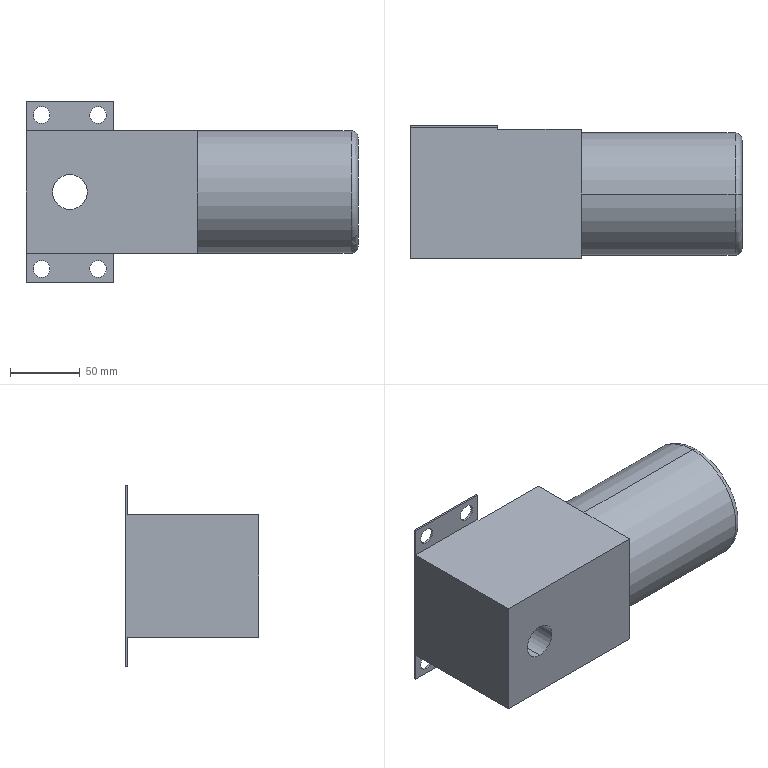Part | SolidWorks | features ICE 5, Extrusion 1, Fillet 1 | 1 solid | 28 faces | box 238.5 x 96 x 130.5 mm | volume 1680517 mm3 | plane 14 | cylinder 12 | torus 2 | commonest cylinder face diameters 12 x8 25 x2 88 x2
STEP:
#1=CARTESIAN_POINT('',(202.,-48.,44.));
#2=VERTEX_POINT('',#1);
#3=CARTESIAN_POINT('',(202.,-48.,-44.));
#4=VERTEX_POINT('',#3);
#5=CARTESIAN_POINT('',(202.,-48.,0.));
#6=DIRECTION('',(-1.,0.,0.));
#7=DIRECTION('',(0.,0.,-1.));
#8=AXIS2_PLACEMENT_3D('',#5,#6,#7);
#9=CIRCLE('',#8,44.);
#10=EDGE_CURVE('',#2,#4,#9,.T.);
#11=ORIENTED_EDGE('',*,*,#10,.F.);
#12=CARTESIAN_POINT('',(207.,-48.,39.));
#13=VERTEX_POINT('',#12);
#14=CARTESIAN_POINT('',(202.,-48.,39.));
#15=DIRECTION('',(0.,1.,0.));
#16=DIRECTION('',(0.,0.,1.));
#17=AXIS2_PLACEMENT_3D('',#14,#15,#16);
#18=CIRCLE('',#17,5.);
#19=EDGE_CURVE('',#2,#13,#18,.T.);
#20=ORIENTED_EDGE('',*,*,#19,.T.);
#21=CARTESIAN_POINT('',(207.,-48.,-39.));
#22=VERTEX_POINT('',#21);
#23=CARTESIAN_POINT('',(207.,-48.,0.));
#24=DIRECTION('',(1.,0.,0.));
#25=DIRECTION('',(0.,0.,-1.));
#26=AXIS2_PLACEMENT_3D('',#23,#24,#25);
#27=CIRCLE('',#26,39.);
#28=EDGE_CURVE('',#22,#13,#27,.T.);
#29=ORIENTED_EDGE('',*,*,#28,.F.);
#30=CARTESIAN_POINT('',(202.,-48.,-39.));
#31=DIRECTION('',(0.,-1.,0.));
#32=DIRECTION('',(0.,0.,-1.));
#33=AXIS2_PLACEMENT_3D('',#30,#31,#32);
#34=CIRCLE('',#33,5.);
#35=EDGE_CURVE('',#4,#22,#34,.T.);
#36=ORIENTED_EDGE('',*,*,#35,.F.);
#37=EDGE_LOOP('',(#11,#20,#29,#36));
#38=FACE_OUTER_BOUND('',#37,.T.);
#39=CARTESIAN_POINT('',(202.,-48.,0.));
#40=DIRECTION('',(1.,0.,0.));
#41=DIRECTION('',(0.,0.,-1.));
#42=AXIS2_PLACEMENT_3D('',#39,#40,#41);
#43=TOROIDAL_SURFACE('',#42,39.,5.);
#44=ADVANCED_FACE('',(#38),#43,.T.);
#45=CARTESIAN_POINT('',(0.,-94.5,-12.5));
#46=VERTEX_POINT('',#45);
#47=CARTESIAN_POINT('',(0.,-94.5,12.5));
#48=VERTEX_POINT('',#47);
#49=CARTESIAN_POINT('',(0.,-94.5,0.));
#50=DIRECTION('',(0.,1.,0.));
#51=DIRECTION('',(0.,0.,1.));
#52=AXIS2_PLACEMENT_3D('',#49,#50,#51);
#53=CIRCLE('',#52,12.5);
#54=EDGE_CURVE('',#46,#48,#53,.T.);
#55=ORIENTED_EDGE('',*,*,#54,.F.);
#56=CARTESIAN_POINT('',(0.,1.5,-12.5));
#57=VERTEX_POINT('',#56);
#58=CARTESIAN_POINT('',(0.,-94.5,-12.5));
#59=DIRECTION('',(0.,1.,0.));
#60=VECTOR('',#59,1000.);
#61=LINE('',#58,#60);
#62=EDGE_CURVE('',#46,#57,#61,.T.);
#63=ORIENTED_EDGE('',*,*,#62,.T.);
#64=CARTESIAN_POINT('',(0.,1.5,12.5));
#65=VERTEX_POINT('',#64);
#66=CARTESIAN_POINT('',(0.,1.5,0.));
#67=DIRECTION('',(0.,1.,0.));
#68=DIRECTION('',(0.,0.,1.));
#69=AXIS2_PLACEMENT_3D('',#66,#67,#68);
#70=CIRCLE('',#69,12.5);
#71=EDGE_CURVE('',#57,#65,#70,.T.);
#72=ORIENTED_EDGE('',*,*,#71,.T.);
#73=CARTESIAN_POINT('',(0.,-94.5,12.5));
#74=DIRECTION('',(0.,1.,0.));
#75=VECTOR('',#74,1000.);
#76=LINE('',#73,#75);
#77=EDGE_CURVE('',#48,#65,#76,.T.);
#78=ORIENTED_EDGE('',*,*,#77,.F.);
#79=EDGE_LOOP('',(#55,#63,#72,#78));
#80=FACE_OUTER_BOUND('',#79,.T.);
#81=CARTESIAN_POINT('',(0.,-94.5,0.));
#82=DIRECTION('',(0.,1.,0.));
#83=DIRECTION('',(0.,0.,1.));
#84=AXIS2_PLACEMENT_3D('',#81,#82,#83);
#85=CYLINDRICAL_SURFACE('',#84,12.5);
#86=ADVANCED_FACE('',(#80),#85,.F.);
#87=CARTESIAN_POINT('',(20.25,0.,49.25));
#88=VERTEX_POINT('',#87);
#89=CARTESIAN_POINT('',(20.25,0.,61.25));
#90=VERTEX_POINT('',#89);
#91=CARTESIAN_POINT('',(20.25,0.,55.25));
#92=DIRECTION('',(0.,1.,0.));
#93=DIRECTION('',(0.,0.,1.));
#94=AXIS2_PLACEMENT_3D('',#91,#92,#93);
#95=CIRCLE('',#94,6.);
#96=EDGE_CURVE('',#88,#90,#95,.T.);
#97=ORIENTED_EDGE('',*,*,#96,.F.);
#98=CARTESIAN_POINT('',(20.25,1.5,49.25));
#99=VERTEX_POINT('',#98);
#100=CARTESIAN_POINT('',(20.25,-94.5,49.25));
#101=DIRECTION('',(0.,1.,0.));
#102=VECTOR('',#101,1000.);
#103=LINE('',#100,#102);
#104=EDGE_CURVE('',#88,#99,#103,.T.);
#105=ORIENTED_EDGE('',*,*,#104,.T.);
#106=CARTESIAN_POINT('',(20.25,1.5,61.25));
#107=VERTEX_POINT('',#106);
#108=CARTESIAN_POINT('',(20.25,1.5,55.25));
#109=DIRECTION('',(0.,1.,0.));
#110=DIRECTION('',(0.,0.,1.));
#111=AXIS2_PLACEMENT_3D('',#108,#109,#110);
#112=CIRCLE('',#111,6.);
#113=EDGE_CURVE('',#99,#107,#112,.T.);
#114=ORIENTED_EDGE('',*,*,#113,.T.);
#115=CARTESIAN_POINT('',(20.25,-94.5,61.25));
#116=DIRECTION('',(0.,1.,0.));
#117=VECTOR('',#116,1000.);
#118=LINE('',#115,#117);
#119=EDGE_CURVE('',#90,#107,#118,.T.);
#120=ORIENTED_EDGE('',*,*,#119,.F.);
#121=EDGE_LOOP('',(#97,#105,#114,#120));
#122=FACE_OUTER_BOUND('',#121,.T.);
#123=CARTESIAN_POINT('',(20.25,-94.5,55.25));
#124=DIRECTION('',(0.,1.,0.));
#125=DIRECTION('',(0.,0.,1.));
#126=AXIS2_PLACEMENT_3D('',#123,#124,#125);
#127=CYLINDRICAL_SURFACE('',#126,6.);
#128=ADVANCED_FACE('',(#122),#127,.F.);
#129=CARTESIAN_POINT('',(-20.25,0.,49.25));
#130=VERTEX_POINT('',#129);
#131=CARTESIAN_POINT('',(-20.25,0.,61.25));
#132=VERTEX_POINT('',#131);
#133=CARTESIAN_POINT('',(-20.25,0.,55.25));
#134=DIRECTION('',(0.,1.,0.));
#135=DIRECTION('',(0.,0.,1.));
#136=AXIS2_PLACEMENT_3D('',#133,#134,#135);
#137=CIRCLE('',#136,6.);
#138=EDGE_CURVE('',#130,#132,#137,.T.);
#139=ORIENTED_EDGE('',*,*,#138,.F.);
#140=CARTESIAN_POINT('',(-20.25,1.5,49.25));
#141=VERTEX_POINT('',#140);
#142=CARTESIAN_POINT('',(-20.25,-94.5,49.25));
#143=DIRECTION('',(0.,1.,0.));
#144=VECTOR('',#143,1000.);
#145=LINE('',#142,#144);
#146=EDGE_CURVE('',#130,#141,#145,.T.);
#147=ORIENTED_EDGE('',*,*,#146,.T.);
#148=CARTESIAN_POINT('',(-20.25,1.5,61.25));
#149=VERTEX_POINT('',#148);
#150=CARTESIAN_POINT('',(-20.25,1.5,55.25));
#151=DIRECTION('',(0.,1.,0.));
#152=DIRECTION('',(0.,0.,1.));
#153=AXIS2_PLACEMENT_3D('',#150,#151,#152);
#154=CIRCLE('',#153,6.);
#155=EDGE_CURVE('',#141,#149,#154,.T.);
#156=ORIENTED_EDGE('',*,*,#155,.T.);
#157=CARTESIAN_POINT('',(-20.25,-94.5,61.25));
#158=DIRECTION('',(0.,1.,0.));
#159=VECTOR('',#158,1000.);
#160=LINE('',#157,#159);
#161=EDGE_CURVE('',#132,#149,#160,.T.);
#162=ORIENTED_EDGE('',*,*,#161,.F.);
#163=EDGE_LOOP('',(#139,#147,#156,#162));
#164=FACE_OUTER_BOUND('',#163,.T.);
#165=CARTESIAN_POINT('',(-20.25,-94.5,55.25));
#166=DIRECTION('',(0.,1.,0.));
#167=DIRECTION('',(0.,0.,1.));
#168=AXIS2_PLACEMENT_3D('',#165,#166,#167);
#169=CYLINDRICAL_SURFACE('',#168,6.);
#170=ADVANCED_FACE('',(#164),#169,.F.);
#171=CARTESIAN_POINT('',(20.25,0.,-61.25));
#172=VERTEX_POINT('',#171);
#173=CARTESIAN_POINT('',(20.25,0.,-49.25));
#174=VERTEX_POINT('',#173);
#175=CARTESIAN_POINT('',(20.25,0.,-55.25));
#176=DIRECTION('',(0.,1.,0.));
#177=DIRECTION('',(0.,0.,1.));
#178=AXIS2_PLACEMENT_3D('',#175,#176,#177);
#179=CIRCLE('',#178,6.);
#180=EDGE_CURVE('',#172,#174,#179,.T.);
#181=ORIENTED_EDGE('',*,*,#180,.F.);
#182=CARTESIAN_POINT('',(20.25,1.5,-61.25));
#183=VERTEX_POINT('',#182);
#184=CARTESIAN_POINT('',(20.25,-94.5,-61.25));
#185=DIRECTION('',(0.,1.,0.));
#186=VECTOR('',#185,1000.);
#187=LINE('',#184,#186);
#188=EDGE_CURVE('',#172,#183,#187,.T.);
#189=ORIENTED_EDGE('',*,*,#188,.T.);
#190=CARTESIAN_POINT('',(20.25,1.5,-49.25));
#191=VERTEX_POINT('',#190);
#192=CARTESIAN_POINT('',(20.25,1.5,-55.25));
#193=DIRECTION('',(0.,1.,0.));
#194=DIRECTION('',(0.,0.,1.));
#195=AXIS2_PLACEMENT_3D('',#192,#193,#194);
#196=CIRCLE('',#195,6.);
#197=EDGE_CURVE('',#183,#191,#196,.T.);
#198=ORIENTED_EDGE('',*,*,#197,.T.);
#199=CARTESIAN_POINT('',(20.25,-94.5,-49.25));
#200=DIRECTION('',(0.,1.,0.));
#201=VECTOR('',#200,1000.);
#202=LINE('',#199,#201);
#203=EDGE_CURVE('',#174,#191,#202,.T.);
#204=ORIENTED_EDGE('',*,*,#203,.F.);
#205=EDGE_LOOP('',(#181,#189,#198,#204));
#206=FACE_OUTER_BOUND('',#205,.T.);
#207=CARTESIAN_POINT('',(20.25,-94.5,-55.25));
#208=DIRECTION('',(0.,1.,0.));
#209=DIRECTION('',(0.,0.,1.));
#210=AXIS2_PLACEMENT_3D('',#207,#208,#209);
#211=CYLINDRICAL_SURFACE('',#210,6.);
#212=ADVANCED_FACE('',(#206),#211,.F.);
#213=CARTESIAN_POINT('',(-20.25,0.,-61.25));
#214=VERTEX_POINT('',#213);
#215=CARTESIAN_POINT('',(-20.25,0.,-49.25));
#216=VERTEX_POINT('',#215);
#217=CARTESIAN_POINT('',(-20.25,0.,-55.25));
#218=DIRECTION('',(0.,1.,0.));
#219=DIRECTION('',(0.,0.,1.));
#220=AXIS2_PLACEMENT_3D('',#217,#218,#219);
#221=CIRCLE('',#220,6.);
#222=EDGE_CURVE('',#214,#216,#221,.T.);
#223=ORIENTED_EDGE('',*,*,#222,.F.);
#224=CARTESIAN_POINT('',(-20.25,1.5,-61.25));
#225=VERTEX_POINT('',#224);
#226=CARTESIAN_POINT('',(-20.25,-94.5,-61.25));
#227=DIRECTION('',(0.,1.,0.));
#228=VECTOR('',#227,1000.);
#229=LINE('',#226,#228);
#230=EDGE_CURVE('',#214,#225,#229,.T.);
#231=ORIENTED_EDGE('',*,*,#230,.T.);
#232=CARTESIAN_POINT('',(-20.25,1.5,-49.25));
#233=VERTEX_POINT('',#232);
#234=CARTESIAN_POINT('',(-20.25,1.5,-55.25));
#235=DIRECTION('',(0.,1.,0.));
#236=DIRECTION('',(0.,0.,1.));
#237=AXIS2_PLACEMENT_3D('',#234,#235,#236);
#238=CIRCLE('',#237,6.);
#239=EDGE_CURVE('',#225,#233,#238,.T.);
#240=ORIENTED_EDGE('',*,*,#239,.T.);
#241=CARTESIAN_POINT('',(-20.25,-94.5,-49.25));
#242=DIRECTION('',(0.,1.,0.));
#243=VECTOR('',#242,1000.);
#244=LINE('',#241,#243);
#245=EDGE_CURVE('',#216,#233,#244,.T.);
#246=ORIENTED_EDGE('',*,*,#245,.F.);
#247=EDGE_LOOP('',(#223,#231,#240,#246));
#248=FACE_OUTER_BOUND('',#247,.T.);
#249=CARTESIAN_POINT('',(-20.25,-94.5,-55.25));
#250=DIRECTION('',(0.,1.,0.));
#251=DIRECTION('',(0.,0.,1.));
#252=AXIS2_PLACEMENT_3D('',#249,#250,#251);
#253=CYLINDRICAL_SURFACE('',#252,6.);
#254=ADVANCED_FACE('',(#248),#253,.F.);
#255=ORIENTED_EDGE('',*,*,#10,.T.);
#256=CARTESIAN_POINT('',(91.5,-48.,-44.));
#257=VERTEX_POINT('',#256);
#258=CARTESIAN_POINT('',(207.,-48.,-44.));
#259=DIRECTION('',(-1.,0.,0.));
#260=VECTOR('',#259,1000.);
#261=LINE('',#258,#260);
#262=EDGE_CURVE('',#4,#257,#261,.T.);
#263=ORIENTED_EDGE('',*,*,#262,.T.);
#264=CARTESIAN_POINT('',(91.5,-48.,44.));
#265=VERTEX_POINT('',#264);
#266=CARTESIAN_POINT('',(91.5,-48.,0.));
#267=DIRECTION('',(1.,0.,0.));
#268=DIRECTION('',(0.,0.,-1.));
#269=AXIS2_PLACEMENT_3D('',#266,#267,#268);
#270=CIRCLE('',#269,44.);
#271=EDGE_CURVE('',#257,#265,#270,.T.);
#272=ORIENTED_EDGE('',*,*,#271,.T.);
#273=CARTESIAN_POINT('',(207.,-48.,44.));
#274=DIRECTION('',(-1.,0.,0.));
#275=VECTOR('',#274,1000.);
#276=LINE('',#273,#275);
#277=EDGE_CURVE('',#2,#265,#276,.T.);
#278=ORIENTED_EDGE('',*,*,#277,.F.);
#279=EDGE_LOOP('',(#255,#263,#272,#278));
#280=FACE_OUTER_BOUND('',#279,.T.);
#281=CARTESIAN_POINT('',(207.,-48.,0.));
#282=DIRECTION('',(-1.,0.,0.));
#283=DIRECTION('',(0.,0.,1.));
#284=AXIS2_PLACEMENT_3D('',#281,#282,#283);
#285=CYLINDRICAL_SURFACE('',#284,44.);
#286=ADVANCED_FACE('',(#280),#285,.T.);
#287=CARTESIAN_POINT('',(31.5,-1.5,-44.));
#288=VERTEX_POINT('',#287);
#289=CARTESIAN_POINT('',(31.5,-1.5,44.));
#290=VERTEX_POINT('',#289);
#291=CARTESIAN_POINT('',(31.5,-1.5,-65.25));
#292=DIRECTION('',(0.,0.,1.));
#293=VECTOR('',#292,1000.);
#294=LINE('',#291,#293);
#295=EDGE_CURVE('',#288,#290,#294,.T.);
#296=ORIENTED_EDGE('',*,*,#295,.F.);
#297=CARTESIAN_POINT('',(31.5,0.,-44.));
#298=VERTEX_POINT('',#297);
#299=CARTESIAN_POINT('',(31.5,-3.,-44.));
#300=DIRECTION('',(0.,1.,0.));
#301=VECTOR('',#300,1000.);
#302=LINE('',#299,#301);
#303=EDGE_CURVE('',#288,#298,#302,.T.);
#304=ORIENTED_EDGE('',*,*,#303,.T.);
#305=CARTESIAN_POINT('',(31.5,0.,-65.25));
#306=VERTEX_POINT('',#305);
#307=CARTESIAN_POINT('',(31.5,0.,-65.25));
#308=DIRECTION('',(0.,0.,-1.));
#309=VECTOR('',#308,1000.);
#310=LINE('',#307,#309);
#311=EDGE_CURVE('',#298,#306,#310,.T.);
#312=ORIENTED_EDGE('',*,*,#311,.T.);
#313=CARTESIAN_POINT('',(31.5,1.5,-65.25));
#314=VERTEX_POINT('',#313);
#315=CARTESIAN_POINT('',(31.5,1.5,-65.25));
#316=DIRECTION('',(0.,-1.,0.));
#317=VECTOR('',#316,1000.);
#318=LINE('',#315,#317);
#319=EDGE_CURVE('',#314,#306,#318,.T.);
#320=ORIENTED_EDGE('',*,*,#319,.F.);
#321=CARTESIAN_POINT('',(31.5,1.5,65.25));
#322=VERTEX_POINT('',#321);
#323=CARTESIAN_POINT('',(31.5,1.5,-65.25));
#324=DIRECTION('',(0.,0.,-1.));
#325=VECTOR('',#324,1000.);
#326=LINE('',#323,#325);
#327=EDGE_CURVE('',#322,#314,#326,.T.);
#328=ORIENTED_EDGE('',*,*,#327,.F.);
#329=CARTESIAN_POINT('',(31.5,0.,65.25));
#330=VERTEX_POINT('',#329);
#331=CARTESIAN_POINT('',(31.5,1.5,65.25));
#332=DIRECTION('',(0.,-1.,0.));
#333=VECTOR('',#332,1000.);
#334=LINE('',#331,#333);
#335=EDGE_CURVE('',#322,#330,#334,.T.);
#336=ORIENTED_EDGE('',*,*,#335,.T.);
#337=CARTESIAN_POINT('',(31.5,0.,44.));
#338=VERTEX_POINT('',#337);
#339=CARTESIAN_POINT('',(31.5,0.,-65.25));
#340=DIRECTION('',(0.,0.,-1.));
#341=VECTOR('',#340,1000.);
#342=LINE('',#339,#341);
#343=EDGE_CURVE('',#330,#338,#342,.T.);
#344=ORIENTED_EDGE('',*,*,#343,.T.);
#345=CARTESIAN_POINT('',(31.5,-3.,44.));
#346=DIRECTION('',(0.,1.,0.));
#347=VECTOR('',#346,1000.);
#348=LINE('',#345,#347);
#349=EDGE_CURVE('',#290,#338,#348,.T.);
#350=ORIENTED_EDGE('',*,*,#349,.F.);
#351=EDGE_LOOP('',(#296,#304,#312,#320,#328,#336,#344,#350));
#352=FACE_OUTER_BOUND('',#351,.T.);
#353=CARTESIAN_POINT('',(31.5,1.5,-65.25));
#354=DIRECTION('',(-1.,0.,0.));
#355=DIRECTION('',(0.,0.,1.));
#356=AXIS2_PLACEMENT_3D('',#353,#354,#355);
#357=PLANE('',#356);
#358=ADVANCED_FACE('',(#352),#357,.F.);
#359=CARTESIAN_POINT('',(20.25,0.,55.25));
#360=DIRECTION('',(0.,1.,0.));
#361=DIRECTION('',(0.,0.,1.));
#362=AXIS2_PLACEMENT_3D('',#359,#360,#361);
#363=CIRCLE('',#362,6.);
#364=EDGE_CURVE('',#90,#88,#363,.T.);
#365=ORIENTED_EDGE('',*,*,#364,.T.);
#366=ORIENTED_EDGE('',*,*,#96,.T.);
#367=EDGE_LOOP('',(#365,#366));
#368=FACE_BOUND('',#367,.T.);
#369=CARTESIAN_POINT('',(-20.25,0.,55.25));
#370=DIRECTION('',(0.,1.,0.));
#371=DIRECTION('',(0.,0.,1.));
#372=AXIS2_PLACEMENT_3D('',#369,#370,#371);
#373=CIRCLE('',#372,6.);
#374=EDGE_CURVE('',#132,#130,#373,.T.);
#375=ORIENTED_EDGE('',*,*,#374,.T.);
#376=ORIENTED_EDGE('',*,*,#138,.T.);
#377=EDGE_LOOP('',(#375,#376));
#378=FACE_BOUND('',#377,.T.);
#379=CARTESIAN_POINT('',(-31.5,0.,44.));
#380=VERTEX_POINT('',#379);
#381=CARTESIAN_POINT('',(-31.5,0.,44.));
#382=DIRECTION('',(-1.,0.,0.));
#383=VECTOR('',#382,1000.);
#384=LINE('',#381,#383);
#385=EDGE_CURVE('',#338,#380,#384,.T.);
#386=ORIENTED_EDGE('',*,*,#385,.F.);
#387=ORIENTED_EDGE('',*,*,#343,.F.);
#388=CARTESIAN_POINT('',(-31.5,0.,65.25));
#389=VERTEX_POINT('',#388);
#390=CARTESIAN_POINT('',(-31.5,0.,65.25));
#391=DIRECTION('',(1.,0.,0.));
#392=VECTOR('',#391,1000.);
#393=LINE('',#390,#392);
#394=EDGE_CURVE('',#389,#330,#393,.T.);
#395=ORIENTED_EDGE('',*,*,#394,.F.);
#396=CARTESIAN_POINT('',(-31.5,0.,-65.25));
#397=DIRECTION('',(0.,0.,1.));
#398=VECTOR('',#397,1000.);
#399=LINE('',#396,#398);
#400=EDGE_CURVE('',#380,#389,#399,.T.);
#401=ORIENTED_EDGE('',*,*,#400,.F.);
#402=EDGE_LOOP('',(#386,#387,#395,#401));
#403=FACE_OUTER_BOUND('',#402,.T.);
#404=CARTESIAN_POINT('',(0.,0.,0.));
#405=DIRECTION('',(0.,1.,0.));
#406=DIRECTION('',(0.,0.,1.));
#407=AXIS2_PLACEMENT_3D('',#404,#405,#406);
#408=PLANE('',#407);
#409=ADVANCED_FACE('',(#368,#378,#403),#408,.F.);
#410=CARTESIAN_POINT('',(20.25,0.,-55.25));
#411=DIRECTION('',(0.,1.,0.));
#412=DIRECTION('',(0.,0.,1.));
#413=AXIS2_PLACEMENT_3D('',#410,#411,#412);
#414=CIRCLE('',#413,6.);
#415=EDGE_CURVE('',#174,#172,#414,.T.);
#416=ORIENTED_EDGE('',*,*,#415,.T.);
#417=ORIENTED_EDGE('',*,*,#180,.T.);
#418=EDGE_LOOP('',(#416,#417));
#419=FACE_BOUND('',#418,.T.);
#420=CARTESIAN_POINT('',(-20.25,0.,-55.25));
#421=DIRECTION('',(0.,1.,0.));
#422=DIRECTION('',(0.,0.,1.));
#423=AXIS2_PLACEMENT_3D('',#420,#421,#422);
#424=CIRCLE('',#423,6.);
#425=EDGE_CURVE('',#216,#214,#424,.T.);
#426=ORIENTED_EDGE('',*,*,#425,.T.);
#427=ORIENTED_EDGE('',*,*,#222,.T.);
#428=EDGE_LOOP('',(#426,#427));
#429=FACE_BOUND('',#428,.T.);
#430=CARTESIAN_POINT('',(-31.5,0.,-44.));
#431=VERTEX_POINT('',#430);
#432=CARTESIAN_POINT('',(-31.5,0.,-44.));
#433=DIRECTION('',(1.,0.,0.));
#434=VECTOR('',#433,1000.);
#435=LINE('',#432,#434);
#436=EDGE_CURVE('',#431,#298,#435,.T.);
#437=ORIENTED_EDGE('',*,*,#436,.F.);
#438=CARTESIAN_POINT('',(-31.5,0.,-65.25));
#439=VERTEX_POINT('',#438);
#440=CARTESIAN_POINT('',(-31.5,0.,-65.25));
#441=DIRECTION('',(0.,0.,1.));
#442=VECTOR('',#441,1000.);
#443=LINE('',#440,#442);
#444=EDGE_CURVE('',#439,#431,#443,.T.);
#445=ORIENTED_EDGE('',*,*,#444,.F.);
#446=CARTESIAN_POINT('',(-31.5,0.,-65.25));
#447=DIRECTION('',(-1.,0.,0.));
#448=VECTOR('',#447,1000.);
#449=LINE('',#446,#448);
#450=EDGE_CURVE('',#306,#439,#449,.T.);
#451=ORIENTED_EDGE('',*,*,#450,.F.);
#452=ORIENTED_EDGE('',*,*,#311,.F.);
#453=EDGE_LOOP('',(#437,#445,#451,#452));
#454=FACE_OUTER_BOUND('',#453,.T.);
#455=CARTESIAN_POINT('',(0.,0.,0.));
#456=DIRECTION('',(0.,1.,0.));
#457=DIRECTION('',(0.,0.,1.));
#458=AXIS2_PLACEMENT_3D('',#455,#456,#457);
#459=PLANE('',#458);
#460=ADVANCED_FACE('',(#419,#429,#454),#459,.F.);
#461=ORIENTED_EDGE('',*,*,#450,.T.);
#462=CARTESIAN_POINT('',(-31.5,1.5,-65.25));
#463=VERTEX_POINT('',#462);
#464=CARTESIAN_POINT('',(-31.5,1.5,-65.25));
#465=DIRECTION('',(0.,-1.,0.));
#466=VECTOR('',#465,1000.);
#467=LINE('',#464,#466);
#468=EDGE_CURVE('',#463,#439,#467,.T.);
#469=ORIENTED_EDGE('',*,*,#468,.F.);
#470=CARTESIAN_POINT('',(-31.5,1.5,-65.25));
#471=DIRECTION('',(-1.,0.,0.));
#472=VECTOR('',#471,1000.);
#473=LINE('',#470,#472);
#474=EDGE_CURVE('',#314,#463,#473,.T.);
#475=ORIENTED_EDGE('',*,*,#474,.F.);
#476=ORIENTED_EDGE('',*,*,#319,.T.);
#477=EDGE_LOOP('',(#461,#469,#475,#476));
#478=FACE_OUTER_BOUND('',#477,.T.);
#479=CARTESIAN_POINT('',(-31.5,1.5,-65.25));
#480=DIRECTION('',(0.,0.,1.));
#481=DIRECTION('',(1.,0.,0.));
#482=AXIS2_PLACEMENT_3D('',#479,#480,#481);
#483=PLANE('',#482);
#484=ADVANCED_FACE('',(#478),#483,.F.);
#485=CARTESIAN_POINT('',(-31.5,-94.5,44.));
#486=VERTEX_POINT('',#485);
#487=CARTESIAN_POINT('',(-31.5,-3.,44.));
#488=DIRECTION('',(0.,1.,0.));
#489=VECTOR('',#488,1000.);
#490=LINE('',#487,#489);
#491=EDGE_CURVE('',#486,#380,#490,.T.);
#492=ORIENTED_EDGE('',*,*,#491,.T.);
#493=ORIENTED_EDGE('',*,*,#400,.T.);
#494=CARTESIAN_POINT('',(-31.5,1.5,65.25));
#495=VERTEX_POINT('',#494);
#496=CARTESIAN_POINT('',(-31.5,1.5,65.25));
#497=DIRECTION('',(0.,-1.,0.));
#498=VECTOR('',#497,1000.);
#499=LINE('',#496,#498);
#500=EDGE_CURVE('',#495,#389,#499,.T.);
#501=ORIENTED_EDGE('',*,*,#500,.F.);
#502=CARTESIAN_POINT('',(-31.5,1.5,-65.25));
#503=DIRECTION('',(0.,0.,1.));
#504=VECTOR('',#503,1000.);
#505=LINE('',#502,#504);
#506=EDGE_CURVE('',#463,#495,#505,.T.);
#507=ORIENTED_EDGE('',*,*,#506,.F.);
#508=ORIENTED_EDGE('',*,*,#468,.T.);
#509=ORIENTED_EDGE('',*,*,#444,.T.);
#510=CARTESIAN_POINT('',(-31.5,-94.5,-44.));
#511=VERTEX_POINT('',#510);
#512=CARTESIAN_POINT('',(-31.5,-3.,-44.));
#513=DIRECTION('',(0.,1.,0.));
#514=VECTOR('',#513,1000.);
#515=LINE('',#512,#514);
#516=EDGE_CURVE('',#511,#431,#515,.T.);
#517=ORIENTED_EDGE('',*,*,#516,.F.);
#518=CARTESIAN_POINT('',(-31.5,-94.5,44.));
#519=DIRECTION('',(0.,0.,-1.));
#520=VECTOR('',#519,1000.);
#521=LINE('',#518,#520);
#522=EDGE_CURVE('',#486,#511,#521,.T.);
#523=ORIENTED_EDGE('',*,*,#522,.F.);
#524=EDGE_LOOP('',(#492,#493,#501,#507,#508,#509,#517,#523));
#525=FACE_OUTER_BOUND('',#524,.T.);
#526=CARTESIAN_POINT('',(-31.5,1.5,-65.25));
#527=DIRECTION('',(1.,0.,0.));
#528=DIRECTION('',(0.,0.,-1.));
#529=AXIS2_PLACEMENT_3D('',#526,#527,#528);
#530=PLANE('',#529);
#531=ADVANCED_FACE('',(#525),#530,.F.);
#532=ORIENTED_EDGE('',*,*,#394,.T.);
#533=ORIENTED_EDGE('',*,*,#335,.F.);
#534=CARTESIAN_POINT('',(-31.5,1.5,65.25));
#535=DIRECTION('',(1.,0.,0.));
#536=VECTOR('',#535,1000.);
#537=LINE('',#534,#536);
#538=EDGE_CURVE('',#495,#322,#537,.T.);
#539=ORIENTED_EDGE('',*,*,#538,.F.);
#540=ORIENTED_EDGE('',*,*,#500,.T.);
#541=EDGE_LOOP('',(#532,#533,#539,#540));
#542=FACE_OUTER_BOUND('',#541,.T.);
#543=CARTESIAN_POINT('',(-31.5,1.5,65.25));
#544=DIRECTION('',(0.,0.,-1.));
#545=DIRECTION('',(-1.,0.,0.));
#546=AXIS2_PLACEMENT_3D('',#543,#544,#545);
#547=PLANE('',#546);
#548=ADVANCED_FACE('',(#542),#547,.F.);
#549=CARTESIAN_POINT('',(0.,1.5,0.));
#550=DIRECTION('',(0.,1.,0.));
#551=DIRECTION('',(0.,0.,1.));
#552=AXIS2_PLACEMENT_3D('',#549,#550,#551);
#553=CIRCLE('',#552,12.5);
#554=EDGE_CURVE('',#65,#57,#553,.T.);
#555=ORIENTED_EDGE('',*,*,#554,.F.);
#556=ORIENTED_EDGE('',*,*,#71,.F.);
#557=EDGE_LOOP('',(#555,#556));
#558=FACE_BOUND('',#557,.T.);
#559=CARTESIAN_POINT('',(20.25,1.5,55.25));
#560=DIRECTION('',(0.,1.,0.));
#561=DIRECTION('',(0.,0.,1.));
#562=AXIS2_PLACEMENT_3D('',#559,#560,#561);
#563=CIRCLE('',#562,6.);
#564=EDGE_CURVE('',#107,#99,#563,.T.);
#565=ORIENTED_EDGE('',*,*,#564,.F.);
#566=ORIENTED_EDGE('',*,*,#113,.F.);
#567=EDGE_LOOP('',(#565,#566));
#568=FACE_BOUND('',#567,.T.);
#569=CARTESIAN_POINT('',(-20.25,1.5,55.25));
#570=DIRECTION('',(0.,1.,0.));
#571=DIRECTION('',(0.,0.,1.));
#572=AXIS2_PLACEMENT_3D('',#569,#570,#571);
#573=CIRCLE('',#572,6.);
#574=EDGE_CURVE('',#149,#141,#573,.T.);
#575=ORIENTED_EDGE('',*,*,#574,.F.);
#576=ORIENTED_EDGE('',*,*,#155,.F.);
#577=EDGE_LOOP('',(#575,#576));
#578=FACE_BOUND('',#577,.T.);
#579=CARTESIAN_POINT('',(20.25,1.5,-55.25));
#580=DIRECTION('',(0.,1.,0.));
#581=DIRECTION('',(0.,0.,1.));
#582=AXIS2_PLACEMENT_3D('',#579,#580,#581);
#583=CIRCLE('',#582,6.);
#584=EDGE_CURVE('',#191,#183,#583,.T.);
#585=ORIENTED_EDGE('',*,*,#584,.F.);
#586=ORIENTED_EDGE('',*,*,#197,.F.);
#587=EDGE_LOOP('',(#585,#586));
#588=FACE_BOUND('',#587,.T.);
#589=CARTESIAN_POINT('',(-20.25,1.5,-55.25));
#590=DIRECTION('',(0.,1.,0.));
#591=DIRECTION('',(0.,0.,1.));
#592=AXIS2_PLACEMENT_3D('',#589,#590,#591);
#593=CIRCLE('',#592,6.);
#594=EDGE_CURVE('',#233,#225,#593,.T.);
#595=ORIENTED_EDGE('',*,*,#594,.F.);
#596=ORIENTED_EDGE('',*,*,#239,.F.);
#597=EDGE_LOOP('',(#595,#596));
#598=FACE_BOUND('',#597,.T.);
#599=ORIENTED_EDGE('',*,*,#327,.T.);
#600=ORIENTED_EDGE('',*,*,#474,.T.);
#601=ORIENTED_EDGE('',*,*,#506,.T.);
#602=ORIENTED_EDGE('',*,*,#538,.T.);
#603=EDGE_LOOP('',(#599,#600,#601,#602));
#604=FACE_OUTER_BOUND('',#603,.T.);
#605=CARTESIAN_POINT('',(0.,1.5,0.));
#606=DIRECTION('',(0.,1.,0.));
#607=DIRECTION('',(0.,0.,1.));
#608=AXIS2_PLACEMENT_3D('',#605,#606,#607);
#609=PLANE('',#608);
#610=ADVANCED_FACE('',(#558,#568,#578,#588,#598,#604),#609,.T.);
#611=ORIENTED_EDGE('',*,*,#303,.F.);
#612=CARTESIAN_POINT('',(91.5,-1.5,-44.));
#613=VERTEX_POINT('',#612);
#614=CARTESIAN_POINT('',(-31.5,-1.5,-44.));
#615=DIRECTION('',(1.,0.,0.));
#616=VECTOR('',#615,1000.);
#617=LINE('',#614,#616);
#618=EDGE_CURVE('',#288,#613,#617,.T.);
#619=ORIENTED_EDGE('',*,*,#618,.T.);
#620=CARTESIAN_POINT('',(91.5,-94.5,-44.));
#621=DIRECTION('',(0.,1.,0.));
#622=VECTOR('',#621,1000.);
#623=LINE('',#620,#622);
#624=EDGE_CURVE('',#257,#613,#623,.T.);
#625=ORIENTED_EDGE('',*,*,#624,.F.);
#626=CARTESIAN_POINT('',(91.5,-94.5,-44.));
#627=VERTEX_POINT('',#626);
#628=CARTESIAN_POINT('',(91.5,-94.5,-44.));
#629=DIRECTION('',(0.,1.,0.));
#630=VECTOR('',#629,1000.);
#631=LINE('',#628,#630);
#632=EDGE_CURVE('',#627,#257,#631,.T.);
#633=ORIENTED_EDGE('',*,*,#632,.F.);
#634=CARTESIAN_POINT('',(-31.5,-94.5,-44.));
#635=DIRECTION('',(1.,0.,0.));
#636=VECTOR('',#635,1000.);
#637=LINE('',#634,#636);
#638=EDGE_CURVE('',#511,#627,#637,.T.);
#639=ORIENTED_EDGE('',*,*,#638,.F.);
#640=ORIENTED_EDGE('',*,*,#516,.T.);
#641=ORIENTED_EDGE('',*,*,#436,.T.);
#642=EDGE_LOOP('',(#611,#619,#625,#633,#639,#640,#641));
#643=FACE_OUTER_BOUND('',#642,.T.);
#644=CARTESIAN_POINT('',(-31.5,-3.,-44.));
#645=DIRECTION('',(0.,0.,1.));
#646=DIRECTION('',(1.,0.,0.));
#647=AXIS2_PLACEMENT_3D('',#644,#645,#646);
#648=PLANE('',#647);
#649=ADVANCED_FACE('',(#643),#648,.F.);
#650=CARTESIAN_POINT('',(91.5,-1.5,44.));
#651=VERTEX_POINT('',#650);
#652=CARTESIAN_POINT('',(-31.5,-1.5,44.));
#653=DIRECTION('',(-1.,0.,0.));
#654=VECTOR('',#653,1000.);
#655=LINE('',#652,#654);
#656=EDGE_CURVE('',#651,#290,#655,.T.);
#657=ORIENTED_EDGE('',*,*,#656,.T.);
#658=ORIENTED_EDGE('',*,*,#349,.T.);
#659=ORIENTED_EDGE('',*,*,#385,.T.);
#660=ORIENTED_EDGE('',*,*,#491,.F.);
#661=CARTESIAN_POINT('',(91.5,-94.5,44.));
#662=VERTEX_POINT('',#661);
#663=CARTESIAN_POINT('',(-31.5,-94.5,44.));
#664=DIRECTION('',(-1.,0.,0.));
#665=VECTOR('',#664,1000.);
#666=LINE('',#663,#665);
#667=EDGE_CURVE('',#662,#486,#666,.T.);
#668=ORIENTED_EDGE('',*,*,#667,.F.);
#669=CARTESIAN_POINT('',(91.5,-94.5,44.));
#670=DIRECTION('',(0.,1.,0.));
#671=VECTOR('',#670,1000.);
#672=LINE('',#669,#671);
#673=EDGE_CURVE('',#662,#265,#672,.T.);
#674=ORIENTED_EDGE('',*,*,#673,.T.);
#675=CARTESIAN_POINT('',(91.5,-94.5,44.));
#676=DIRECTION('',(0.,1.,0.));
#677=VECTOR('',#676,1000.);
#678=LINE('',#675,#677);
#679=EDGE_CURVE('',#265,#651,#678,.T.);
#680=ORIENTED_EDGE('',*,*,#679,.T.);
#681=EDGE_LOOP('',(#657,#658,#659,#660,#668,#674,#680));
#682=FACE_OUTER_BOUND('',#681,.T.);
#683=CARTESIAN_POINT('',(-31.5,-3.,44.));
#684=DIRECTION('',(0.,0.,-1.));
#685=DIRECTION('',(-1.,0.,0.));
#686=AXIS2_PLACEMENT_3D('',#683,#684,#685);
#687=PLANE('',#686);
#688=ADVANCED_FACE('',(#682),#687,.F.);
#689=ORIENTED_EDGE('',*,*,#618,.F.);
#690=ORIENTED_EDGE('',*,*,#295,.T.);
#691=ORIENTED_EDGE('',*,*,#656,.F.);
#692=CARTESIAN_POINT('',(91.5,-1.5,44.));
#693=DIRECTION('',(0.,0.,1.));
#694=VECTOR('',#693,1000.);
#695=LINE('',#692,#694);
#696=EDGE_CURVE('',#613,#651,#695,.T.);
#697=ORIENTED_EDGE('',*,*,#696,.F.);
#698=EDGE_LOOP('',(#689,#690,#691,#697));
#699=FACE_OUTER_BOUND('',#698,.T.);
#700=CARTESIAN_POINT('',(0.,-1.5,0.));
#701=DIRECTION('',(0.,-1.,0.));
#702=DIRECTION('',(0.,0.,-1.));
#703=AXIS2_PLACEMENT_3D('',#700,#701,#702);
#704=PLANE('',#703);
#705=ADVANCED_FACE('',(#699),#704,.F.);
#706=ORIENTED_EDGE('',*,*,#271,.F.);
#707=ORIENTED_EDGE('',*,*,#624,.T.);
#708=ORIENTED_EDGE('',*,*,#696,.T.);
#709=ORIENTED_EDGE('',*,*,#679,.F.);
#710=EDGE_LOOP('',(#706,#707,#708,#709));
#711=FACE_OUTER_BOUND('',#710,.T.);
#712=CARTESIAN_POINT('',(91.5,-94.5,44.));
#713=DIRECTION('',(-1.,0.,0.));
#714=DIRECTION('',(0.,0.,1.));
#715=AXIS2_PLACEMENT_3D('',#712,#713,#714);
#716=PLANE('',#715);
#717=ADVANCED_FACE('',(#711),#716,.F.);
#718=CARTESIAN_POINT('',(91.5,-48.,0.));
#719=DIRECTION('',(1.,0.,0.));
#720=DIRECTION('',(0.,0.,-1.));
#721=AXIS2_PLACEMENT_3D('',#718,#719,#720);
#722=CIRCLE('',#721,44.);
#723=EDGE_CURVE('',#265,#257,#722,.T.);
#724=ORIENTED_EDGE('',*,*,#723,.F.);
#725=ORIENTED_EDGE('',*,*,#673,.F.);
#726=CARTESIAN_POINT('',(91.5,-94.5,44.));
#727=DIRECTION('',(0.,0.,1.));
#728=VECTOR('',#727,1000.);
#729=LINE('',#726,#728);
#730=EDGE_CURVE('',#627,#662,#729,.T.);
#731=ORIENTED_EDGE('',*,*,#730,.F.);
#732=ORIENTED_EDGE('',*,*,#632,.T.);
#733=EDGE_LOOP('',(#724,#725,#731,#732));
#734=FACE_OUTER_BOUND('',#733,.T.);
#735=CARTESIAN_POINT('',(91.5,-94.5,44.));
#736=DIRECTION('',(-1.,0.,0.));
#737=DIRECTION('',(0.,0.,1.));
#738=AXIS2_PLACEMENT_3D('',#735,#736,#737);
#739=PLANE('',#738);
#740=ADVANCED_FACE('',(#734),#739,.F.);
#741=CARTESIAN_POINT('',(0.,-94.5,0.));
#742=DIRECTION('',(0.,1.,0.));
#743=DIRECTION('',(0.,0.,1.));
#744=AXIS2_PLACEMENT_3D('',#741,#742,#743);
#745=CIRCLE('',#744,12.5);
#746=EDGE_CURVE('',#48,#46,#745,.T.);
#747=ORIENTED_EDGE('',*,*,#746,.T.);
#748=ORIENTED_EDGE('',*,*,#54,.T.);
#749=EDGE_LOOP('',(#747,#748));
#750=FACE_BOUND('',#749,.T.);
#751=ORIENTED_EDGE('',*,*,#522,.T.);
#752=ORIENTED_EDGE('',*,*,#638,.T.);
#753=ORIENTED_EDGE('',*,*,#730,.T.);
#754=ORIENTED_EDGE('',*,*,#667,.T.);
#755=EDGE_LOOP('',(#751,#752,#753,#754));
#756=FACE_OUTER_BOUND('',#755,.T.);
#757=CARTESIAN_POINT('',(0.,-94.5,0.));
#758=DIRECTION('',(0.,-1.,0.));
#759=DIRECTION('',(0.,0.,-1.));
#760=AXIS2_PLACEMENT_3D('',#757,#758,#759);
#761=PLANE('',#760);
#762=ADVANCED_FACE('',(#750,#756),#761,.T.);
#763=ORIENTED_EDGE('',*,*,#262,.F.);
#764=CARTESIAN_POINT('',(202.,-48.,0.));
#765=DIRECTION('',(-1.,0.,0.));
#766=DIRECTION('',(0.,0.,-1.));
#767=AXIS2_PLACEMENT_3D('',#764,#765,#766);
#768=CIRCLE('',#767,44.);
#769=EDGE_CURVE('',#4,#2,#768,.T.);
#770=ORIENTED_EDGE('',*,*,#769,.T.);
#771=ORIENTED_EDGE('',*,*,#277,.T.);
#772=ORIENTED_EDGE('',*,*,#723,.T.);
#773=EDGE_LOOP('',(#763,#770,#771,#772));
#774=FACE_OUTER_BOUND('',#773,.T.);
#775=CARTESIAN_POINT('',(207.,-48.,0.));
#776=DIRECTION('',(-1.,0.,0.));
#777=DIRECTION('',(0.,0.,1.));
#778=AXIS2_PLACEMENT_3D('',#775,#776,#777);
#779=CYLINDRICAL_SURFACE('',#778,44.);
#780=ADVANCED_FACE('',(#774),#779,.T.);
#781=ORIENTED_EDGE('',*,*,#28,.T.);
#782=CARTESIAN_POINT('',(207.,-48.,0.));
#783=DIRECTION('',(1.,0.,0.));
#784=DIRECTION('',(0.,0.,-1.));
#785=AXIS2_PLACEMENT_3D('',#782,#783,#784);
#786=CIRCLE('',#785,39.);
#787=EDGE_CURVE('',#13,#22,#786,.T.);
#788=ORIENTED_EDGE('',*,*,#787,.T.);
#789=EDGE_LOOP('',(#781,#788));
#790=FACE_OUTER_BOUND('',#789,.T.);
#791=CARTESIAN_POINT('',(207.,-48.,0.));
#792=DIRECTION('',(1.,0.,0.));
#793=DIRECTION('',(0.,0.,-1.));
#794=AXIS2_PLACEMENT_3D('',#791,#792,#793);
#795=PLANE('',#794);
#796=ADVANCED_FACE('',(#790),#795,.T.);
#797=ORIENTED_EDGE('',*,*,#230,.F.);
#798=ORIENTED_EDGE('',*,*,#425,.F.);
#799=ORIENTED_EDGE('',*,*,#245,.T.);
#800=ORIENTED_EDGE('',*,*,#594,.T.);
#801=EDGE_LOOP('',(#797,#798,#799,#800));
#802=FACE_OUTER_BOUND('',#801,.T.);
#803=CARTESIAN_POINT('',(-20.25,-94.5,-55.25));
#804=DIRECTION('',(0.,1.,0.));
#805=DIRECTION('',(0.,0.,1.));
#806=AXIS2_PLACEMENT_3D('',#803,#804,#805);
#807=CYLINDRICAL_SURFACE('',#806,6.);
#808=ADVANCED_FACE('',(#802),#807,.F.);
#809=ORIENTED_EDGE('',*,*,#188,.F.);
#810=ORIENTED_EDGE('',*,*,#415,.F.);
#811=ORIENTED_EDGE('',*,*,#203,.T.);
#812=ORIENTED_EDGE('',*,*,#584,.T.);
#813=EDGE_LOOP('',(#809,#810,#811,#812));
#814=FACE_OUTER_BOUND('',#813,.T.);
#815=CARTESIAN_POINT('',(20.25,-94.5,-55.25));
#816=DIRECTION('',(0.,1.,0.));
#817=DIRECTION('',(0.,0.,1.));
#818=AXIS2_PLACEMENT_3D('',#815,#816,#817);
#819=CYLINDRICAL_SURFACE('',#818,6.);
#820=ADVANCED_FACE('',(#814),#819,.F.);
#821=ORIENTED_EDGE('',*,*,#146,.F.);
#822=ORIENTED_EDGE('',*,*,#374,.F.);
#823=ORIENTED_EDGE('',*,*,#161,.T.);
#824=ORIENTED_EDGE('',*,*,#574,.T.);
#825=EDGE_LOOP('',(#821,#822,#823,#824));
#826=FACE_OUTER_BOUND('',#825,.T.);
#827=CARTESIAN_POINT('',(-20.25,-94.5,55.25));
#828=DIRECTION('',(0.,1.,0.));
#829=DIRECTION('',(0.,0.,1.));
#830=AXIS2_PLACEMENT_3D('',#827,#828,#829);
#831=CYLINDRICAL_SURFACE('',#830,6.);
#832=ADVANCED_FACE('',(#826),#831,.F.);
#833=ORIENTED_EDGE('',*,*,#104,.F.);
#834=ORIENTED_EDGE('',*,*,#364,.F.);
#835=ORIENTED_EDGE('',*,*,#119,.T.);
#836=ORIENTED_EDGE('',*,*,#564,.T.);
#837=EDGE_LOOP('',(#833,#834,#835,#836));
#838=FACE_OUTER_BOUND('',#837,.T.);
#839=CARTESIAN_POINT('',(20.25,-94.5,55.25));
#840=DIRECTION('',(0.,1.,0.));
#841=DIRECTION('',(0.,0.,1.));
#842=AXIS2_PLACEMENT_3D('',#839,#840,#841);
#843=CYLINDRICAL_SURFACE('',#842,6.);
#844=ADVANCED_FACE('',(#838),#843,.F.);
#845=ORIENTED_EDGE('',*,*,#62,.F.);
#846=ORIENTED_EDGE('',*,*,#746,.F.);
#847=ORIENTED_EDGE('',*,*,#77,.T.);
#848=ORIENTED_EDGE('',*,*,#554,.T.);
#849=EDGE_LOOP('',(#845,#846,#847,#848));
#850=FACE_OUTER_BOUND('',#849,.T.);
#851=CARTESIAN_POINT('',(0.,-94.5,0.));
#852=DIRECTION('',(0.,1.,0.));
#853=DIRECTION('',(0.,0.,1.));
#854=AXIS2_PLACEMENT_3D('',#851,#852,#853);
#855=CYLINDRICAL_SURFACE('',#854,12.5);
#856=ADVANCED_FACE('',(#850),#855,.F.);
#857=ORIENTED_EDGE('',*,*,#19,.F.);
#858=ORIENTED_EDGE('',*,*,#769,.F.);
#859=ORIENTED_EDGE('',*,*,#35,.T.);
#860=ORIENTED_EDGE('',*,*,#787,.F.);
#861=EDGE_LOOP('',(#857,#858,#859,#860));
#862=FACE_OUTER_BOUND('',#861,.T.);
#863=CARTESIAN_POINT('',(202.,-48.,0.));
#864=DIRECTION('',(1.,0.,0.));
#865=DIRECTION('',(0.,0.,-1.));
#866=AXIS2_PLACEMENT_3D('',#863,#864,#865);
#867=TOROIDAL_SURFACE('',#866,39.,5.);
#868=ADVANCED_FACE('',(#862),#867,.T.);
#869=CLOSED_SHELL('',(#44,#86,#128,#170,#212,#254,#286,#358,#409,#460,#484,#531,#548,#610,#649,#688,#705,#717,#740,#762,#780,#796,#808,#820,#832,#844,#856,#868));
#870=MANIFOLD_SOLID_BREP('',#869);
#871=CARTESIAN_POINT('',(0.,0.,0.));
#872=DIRECTION('',(0.,0.,1.));
#873=DIRECTION('',(1.,0.,0.));
#874=AXIS2_PLACEMENT_3D('',#871,#872,#873);
#875=(LENGTH_UNIT()NAMED_UNIT(*)SI_UNIT(.MILLI.,.METRE.));
#876=UNCERTAINTY_MEASURE_WITH_UNIT(LENGTH_MEASURE(0.00001),#875,'','');
#877=(NAMED_UNIT(*)PLANE_ANGLE_UNIT()SI_UNIT($,.RADIAN.));
#878=(NAMED_UNIT(*)SI_UNIT($,.STERADIAN.)SOLID_ANGLE_UNIT());
#879=(GEOMETRIC_REPRESENTATION_CONTEXT(3)GLOBAL_UNCERTAINTY_ASSIGNED_CONTEXT((#876))GLOBAL_UNIT_ASSIGNED_CONTEXT((#875,#877,#878))REPRESENTATION_CONTEXT('',''));
#880=ADVANCED_BREP_SHAPE_REPRESENTATION('',(#870,#874),#879);